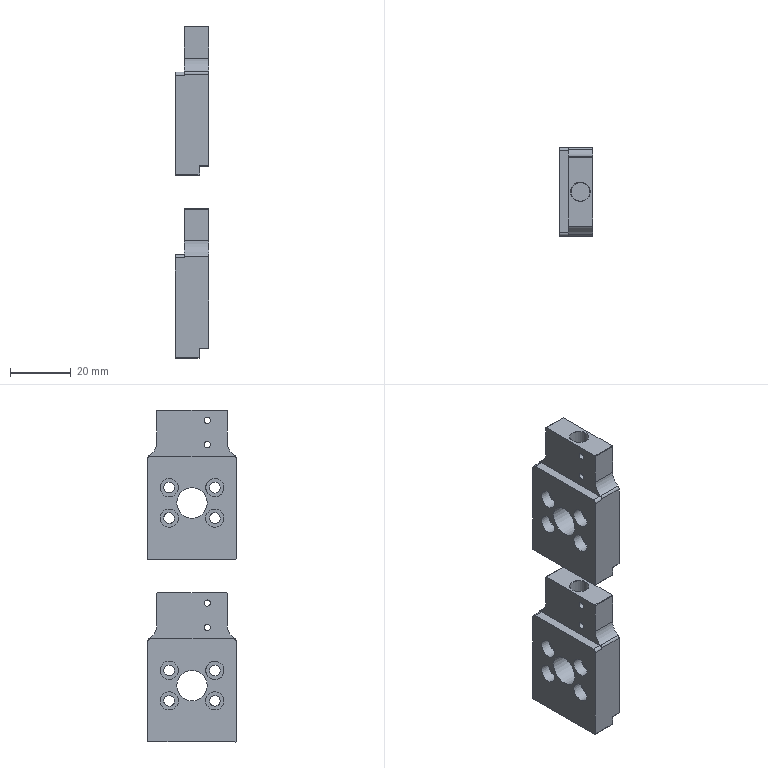Part | 2 solids | 112 faces | box 11 x 29 x 109 mm | volume 18939 mm3 | plane 64 | cylinder 46 | cone 2 | commonest cylinder face diameters 2 x8 3.5 x8 6 x8 3.3 x6 10 x6 2.1 x4